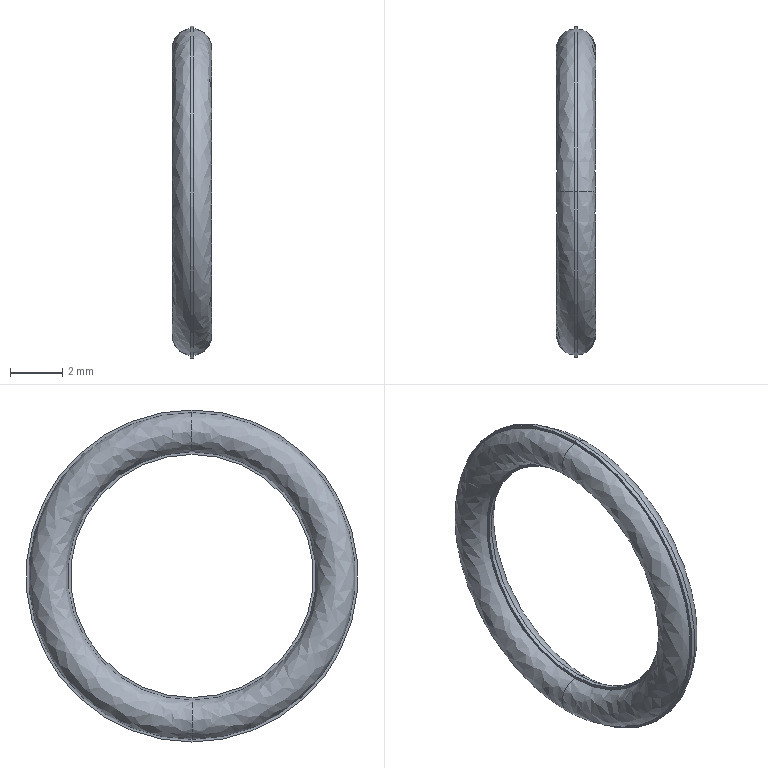Part | SolidWorks | features BaseBody 1 | 1 solid | 12 faces | box 1.5 x 12.7 x 12.7 mm | volume 62.118 mm3 | spline 4 | cylinder 4 | plane 4 | commonest cylinder face diameters 9.3 x2 12.7 x2
STEP:
#1=CARTESIAN_POINT('',(0.075,0.,-4.754));
#2=VERTEX_POINT('',#1);
#3=CARTESIAN_POINT('',(0.075,0.,4.754));
#4=VERTEX_POINT('',#3);
#5=CARTESIAN_POINT('',(0.075,0.,0.));
#6=DIRECTION('',(-1.,0.,0.));
#7=DIRECTION('',(0.,0.,-1.));
#8=AXIS2_PLACEMENT_3D('',#5,#6,#7);
#9=CIRCLE('',#8,4.754);
#10=EDGE_CURVE('',#2,#4,#9,.T.);
#11=ORIENTED_EDGE('',*,*,#10,.T.);
#12=CARTESIAN_POINT('',(0.075,0.,6.246));
#13=VERTEX_POINT('',#12);
#14=CARTESIAN_POINT('',(0.,0.,5.5));
#15=DIRECTION('',(0.,-1.,0.));
#16=DIRECTION('',(0.,0.,1.));
#17=AXIS2_PLACEMENT_3D('',#14,#15,#16);
#18=CIRCLE('',#17,0.75);
#19=EDGE_CURVE('',#4,#13,#18,.T.);
#20=ORIENTED_EDGE('',*,*,#19,.T.);
#21=CARTESIAN_POINT('',(0.075,0.,-6.246));
#22=VERTEX_POINT('',#21);
#23=CARTESIAN_POINT('',(0.075,0.,0.));
#24=DIRECTION('',(1.,0.,0.));
#25=DIRECTION('',(0.,0.,-1.));
#26=AXIS2_PLACEMENT_3D('',#23,#24,#25);
#27=CIRCLE('',#26,6.246);
#28=EDGE_CURVE('',#13,#22,#27,.T.);
#29=ORIENTED_EDGE('',*,*,#28,.T.);
#30=CARTESIAN_POINT('',(0.,0.,-5.5));
#31=DIRECTION('',(0.,1.,0.));
#32=DIRECTION('',(0.,0.,-1.));
#33=AXIS2_PLACEMENT_3D('',#30,#31,#32);
#34=CIRCLE('',#33,0.75);
#35=EDGE_CURVE('',#2,#22,#34,.T.);
#36=ORIENTED_EDGE('',*,*,#35,.F.);
#37=EDGE_LOOP('',(#11,#20,#29,#36));
#38=FACE_OUTER_BOUND('',#37,.T.);
#39=CARTESIAN_POINT('',(0.075,0.,4.754));
#40=CARTESIAN_POINT('',(0.075,-9.508,4.754));
#41=CARTESIAN_POINT('',(0.075,-9.508,-4.754));
#42=CARTESIAN_POINT('',(0.075,0.,-4.754));
#43=CARTESIAN_POINT('',(1.313,0.,4.878));
#44=CARTESIAN_POINT('',(1.313,-9.756,4.878));
#45=CARTESIAN_POINT('',(1.313,-9.756,-4.878));
#46=CARTESIAN_POINT('',(1.313,0.,-4.878));
#47=CARTESIAN_POINT('',(1.313,0.,6.122));
#48=CARTESIAN_POINT('',(1.313,-12.244,6.122));
#49=CARTESIAN_POINT('',(1.313,-12.244,-6.122));
#50=CARTESIAN_POINT('',(1.313,0.,-6.122));
#51=CARTESIAN_POINT('',(0.075,0.,6.246));
#52=CARTESIAN_POINT('',(0.075,-12.492,6.246));
#53=CARTESIAN_POINT('',(0.075,-12.492,-6.246));
#54=CARTESIAN_POINT('',(0.075,0.,-6.246));
#55=(BOUNDED_SURFACE()B_SPLINE_SURFACE(3,3,((#39,#40,#41,#42),(#43,#44,#45,#46),(#47,#48,#49,#50),(#51,#52,#53,#54)),.UNSPECIFIED.,.F.,.F.,.F.)B_SPLINE_SURFACE_WITH_KNOTS((4,4),(4,4),(0.,1.),(0.,1.),.UNSPECIFIED.)GEOMETRIC_REPRESENTATION_ITEM()RATIONAL_B_SPLINE_SURFACE(((1.,0.3333,0.3333,1.),(0.4,0.1333,0.1333,0.4),(0.4,0.1333,0.1333,0.4),(1.,0.3333,0.3333,1.)))REPRESENTATION_ITEM('')SURFACE());
#56=ADVANCED_FACE('',(#38),#55,.T.);
#57=CARTESIAN_POINT('',(-0.075,0.,6.246));
#58=VERTEX_POINT('',#57);
#59=CARTESIAN_POINT('',(-0.075,0.,-6.246));
#60=VERTEX_POINT('',#59);
#61=CARTESIAN_POINT('',(-0.075,0.,0.));
#62=DIRECTION('',(1.,0.,0.));
#63=DIRECTION('',(0.,0.,-1.));
#64=AXIS2_PLACEMENT_3D('',#61,#62,#63);
#65=CIRCLE('',#64,6.246);
#66=EDGE_CURVE('',#58,#60,#65,.T.);
#67=ORIENTED_EDGE('',*,*,#66,.F.);
#68=CARTESIAN_POINT('',(-0.075,0.,4.754));
#69=VERTEX_POINT('',#68);
#70=CARTESIAN_POINT('',(0.,0.,5.5));
#71=DIRECTION('',(0.,-1.,0.));
#72=DIRECTION('',(0.,0.,1.));
#73=AXIS2_PLACEMENT_3D('',#70,#71,#72);
#74=CIRCLE('',#73,0.75);
#75=EDGE_CURVE('',#58,#69,#74,.T.);
#76=ORIENTED_EDGE('',*,*,#75,.T.);
#77=CARTESIAN_POINT('',(-0.075,0.,-4.754));
#78=VERTEX_POINT('',#77);
#79=CARTESIAN_POINT('',(-0.075,0.,0.));
#80=DIRECTION('',(-1.,0.,0.));
#81=DIRECTION('',(0.,0.,-1.));
#82=AXIS2_PLACEMENT_3D('',#79,#80,#81);
#83=CIRCLE('',#82,4.754);
#84=EDGE_CURVE('',#78,#69,#83,.T.);
#85=ORIENTED_EDGE('',*,*,#84,.F.);
#86=CARTESIAN_POINT('',(0.,0.,-5.5));
#87=DIRECTION('',(0.,1.,0.));
#88=DIRECTION('',(0.,0.,-1.));
#89=AXIS2_PLACEMENT_3D('',#86,#87,#88);
#90=CIRCLE('',#89,0.75);
#91=EDGE_CURVE('',#60,#78,#90,.T.);
#92=ORIENTED_EDGE('',*,*,#91,.F.);
#93=EDGE_LOOP('',(#67,#76,#85,#92));
#94=FACE_OUTER_BOUND('',#93,.T.);
#95=CARTESIAN_POINT('',(-0.075,0.,6.246));
#96=CARTESIAN_POINT('',(-0.075,-12.492,6.246));
#97=CARTESIAN_POINT('',(-0.075,-12.492,-6.246));
#98=CARTESIAN_POINT('',(-0.075,0.,-6.246));
#99=CARTESIAN_POINT('',(-1.313,0.,6.122));
#100=CARTESIAN_POINT('',(-1.313,-12.244,6.122));
#101=CARTESIAN_POINT('',(-1.313,-12.244,-6.122));
#102=CARTESIAN_POINT('',(-1.313,0.,-6.122));
#103=CARTESIAN_POINT('',(-1.313,0.,4.878));
#104=CARTESIAN_POINT('',(-1.313,-9.756,4.878));
#105=CARTESIAN_POINT('',(-1.313,-9.756,-4.878));
#106=CARTESIAN_POINT('',(-1.313,0.,-4.878));
#107=CARTESIAN_POINT('',(-0.075,0.,4.754));
#108=CARTESIAN_POINT('',(-0.075,-9.508,4.754));
#109=CARTESIAN_POINT('',(-0.075,-9.508,-4.754));
#110=CARTESIAN_POINT('',(-0.075,0.,-4.754));
#111=(BOUNDED_SURFACE()B_SPLINE_SURFACE(3,3,((#95,#96,#97,#98),(#99,#100,#101,#102),(#103,#104,#105,#106),(#107,#108,#109,#110)),.UNSPECIFIED.,.F.,.F.,.F.)B_SPLINE_SURFACE_WITH_KNOTS((4,4),(4,4),(0.,1.),(0.,1.),.UNSPECIFIED.)GEOMETRIC_REPRESENTATION_ITEM()RATIONAL_B_SPLINE_SURFACE(((1.,0.3333,0.3333,1.),(0.4,0.1333,0.1333,0.4),(0.4,0.1333,0.1333,0.4),(1.,0.3333,0.3333,1.)))REPRESENTATION_ITEM('')SURFACE());
#112=ADVANCED_FACE('',(#94),#111,.T.);
#113=CARTESIAN_POINT('',(0.075,0.,-4.65));
#114=VERTEX_POINT('',#113);
#115=CARTESIAN_POINT('',(0.075,0.,4.65));
#116=VERTEX_POINT('',#115);
#117=CARTESIAN_POINT('',(0.075,0.,0.));
#118=DIRECTION('',(-1.,0.,0.));
#119=DIRECTION('',(0.,0.,1.));
#120=AXIS2_PLACEMENT_3D('',#117,#118,#119);
#121=CIRCLE('',#120,4.65);
#122=EDGE_CURVE('',#114,#116,#121,.T.);
#123=ORIENTED_EDGE('',*,*,#122,.F.);
#124=CARTESIAN_POINT('',(-0.075,0.,-4.65));
#125=VERTEX_POINT('',#124);
#126=CARTESIAN_POINT('',(1.5,0.,-4.65));
#127=DIRECTION('',(-1.,0.,0.));
#128=VECTOR('',#127,1000.);
#129=LINE('',#126,#128);
#130=EDGE_CURVE('',#114,#125,#129,.T.);
#131=ORIENTED_EDGE('',*,*,#130,.T.);
#132=CARTESIAN_POINT('',(-0.075,0.,4.65));
#133=VERTEX_POINT('',#132);
#134=CARTESIAN_POINT('',(-0.075,0.,0.));
#135=DIRECTION('',(1.,0.,0.));
#136=DIRECTION('',(0.,0.,1.));
#137=AXIS2_PLACEMENT_3D('',#134,#135,#136);
#138=CIRCLE('',#137,4.65);
#139=EDGE_CURVE('',#133,#125,#138,.T.);
#140=ORIENTED_EDGE('',*,*,#139,.F.);
#141=CARTESIAN_POINT('',(1.5,0.,4.65));
#142=DIRECTION('',(-1.,0.,0.));
#143=VECTOR('',#142,1000.);
#144=LINE('',#141,#143);
#145=EDGE_CURVE('',#116,#133,#144,.T.);
#146=ORIENTED_EDGE('',*,*,#145,.F.);
#147=EDGE_LOOP('',(#123,#131,#140,#146));
#148=FACE_OUTER_BOUND('',#147,.T.);
#149=CARTESIAN_POINT('',(1.5,0.,0.));
#150=DIRECTION('',(-1.,0.,0.));
#151=DIRECTION('',(0.,0.,1.));
#152=AXIS2_PLACEMENT_3D('',#149,#150,#151);
#153=CYLINDRICAL_SURFACE('',#152,4.65);
#154=ADVANCED_FACE('',(#148),#153,.F.);
#155=CARTESIAN_POINT('',(0.075,0.,-6.35));
#156=VERTEX_POINT('',#155);
#157=CARTESIAN_POINT('',(0.075,0.,6.35));
#158=VERTEX_POINT('',#157);
#159=CARTESIAN_POINT('',(0.075,0.,0.));
#160=DIRECTION('',(1.,0.,0.));
#161=DIRECTION('',(0.,0.,1.));
#162=AXIS2_PLACEMENT_3D('',#159,#160,#161);
#163=CIRCLE('',#162,6.35);
#164=EDGE_CURVE('',#156,#158,#163,.T.);
#165=ORIENTED_EDGE('',*,*,#164,.F.);
#166=CARTESIAN_POINT('',(-0.075,0.,-6.35));
#167=VERTEX_POINT('',#166);
#168=CARTESIAN_POINT('',(1.5,0.,-6.35));
#169=DIRECTION('',(-1.,0.,0.));
#170=VECTOR('',#169,1000.);
#171=LINE('',#168,#170);
#172=EDGE_CURVE('',#156,#167,#171,.T.);
#173=ORIENTED_EDGE('',*,*,#172,.T.);
#174=CARTESIAN_POINT('',(-0.075,0.,6.35));
#175=VERTEX_POINT('',#174);
#176=CARTESIAN_POINT('',(-0.075,0.,0.));
#177=DIRECTION('',(1.,0.,0.));
#178=DIRECTION('',(0.,0.,1.));
#179=AXIS2_PLACEMENT_3D('',#176,#177,#178);
#180=CIRCLE('',#179,6.35);
#181=EDGE_CURVE('',#167,#175,#180,.T.);
#182=ORIENTED_EDGE('',*,*,#181,.T.);
#183=CARTESIAN_POINT('',(1.5,0.,6.35));
#184=DIRECTION('',(-1.,0.,0.));
#185=VECTOR('',#184,1000.);
#186=LINE('',#183,#185);
#187=EDGE_CURVE('',#158,#175,#186,.T.);
#188=ORIENTED_EDGE('',*,*,#187,.F.);
#189=EDGE_LOOP('',(#165,#173,#182,#188));
#190=FACE_OUTER_BOUND('',#189,.T.);
#191=CARTESIAN_POINT('',(1.5,0.,0.));
#192=DIRECTION('',(-1.,0.,0.));
#193=DIRECTION('',(0.,0.,1.));
#194=AXIS2_PLACEMENT_3D('',#191,#192,#193);
#195=CYLINDRICAL_SURFACE('',#194,6.35);
#196=ADVANCED_FACE('',(#190),#195,.T.);
#197=ORIENTED_EDGE('',*,*,#19,.F.);
#198=CARTESIAN_POINT('',(0.075,0.,0.));
#199=DIRECTION('',(-1.,0.,0.));
#200=DIRECTION('',(0.,0.,-1.));
#201=AXIS2_PLACEMENT_3D('',#198,#199,#200);
#202=CIRCLE('',#201,4.754);
#203=EDGE_CURVE('',#4,#2,#202,.T.);
#204=ORIENTED_EDGE('',*,*,#203,.T.);
#205=ORIENTED_EDGE('',*,*,#35,.T.);
#206=CARTESIAN_POINT('',(0.075,0.,0.));
#207=DIRECTION('',(1.,0.,0.));
#208=DIRECTION('',(0.,0.,-1.));
#209=AXIS2_PLACEMENT_3D('',#206,#207,#208);
#210=CIRCLE('',#209,6.246);
#211=EDGE_CURVE('',#22,#13,#210,.T.);
#212=ORIENTED_EDGE('',*,*,#211,.T.);
#213=EDGE_LOOP('',(#197,#204,#205,#212));
#214=FACE_OUTER_BOUND('',#213,.T.);
#215=CARTESIAN_POINT('',(0.075,0.,-4.754));
#216=CARTESIAN_POINT('',(0.075,9.508,-4.754));
#217=CARTESIAN_POINT('',(0.075,9.508,4.754));
#218=CARTESIAN_POINT('',(0.075,0.,4.754));
#219=CARTESIAN_POINT('',(1.313,0.,-4.878));
#220=CARTESIAN_POINT('',(1.313,9.756,-4.878));
#221=CARTESIAN_POINT('',(1.313,9.756,4.878));
#222=CARTESIAN_POINT('',(1.313,0.,4.878));
#223=CARTESIAN_POINT('',(1.313,0.,-6.122));
#224=CARTESIAN_POINT('',(1.313,12.244,-6.122));
#225=CARTESIAN_POINT('',(1.313,12.244,6.122));
#226=CARTESIAN_POINT('',(1.313,0.,6.122));
#227=CARTESIAN_POINT('',(0.075,0.,-6.246));
#228=CARTESIAN_POINT('',(0.075,12.492,-6.246));
#229=CARTESIAN_POINT('',(0.075,12.492,6.246));
#230=CARTESIAN_POINT('',(0.075,0.,6.246));
#231=(BOUNDED_SURFACE()B_SPLINE_SURFACE(3,3,((#215,#216,#217,#218),(#219,#220,#221,#222),(#223,#224,#225,#226),(#227,#228,#229,#230)),.UNSPECIFIED.,.F.,.F.,.F.)B_SPLINE_SURFACE_WITH_KNOTS((4,4),(4,4),(0.,1.),(0.,1.),.UNSPECIFIED.)GEOMETRIC_REPRESENTATION_ITEM()RATIONAL_B_SPLINE_SURFACE(((1.,0.3333,0.3333,1.),(0.4,0.1333,0.1333,0.4),(0.4,0.1333,0.1333,0.4),(1.,0.3333,0.3333,1.)))REPRESENTATION_ITEM('')SURFACE());
#232=ADVANCED_FACE('',(#214),#231,.T.);
#233=CARTESIAN_POINT('',(0.075,0.,0.));
#234=DIRECTION('',(-1.,0.,0.));
#235=DIRECTION('',(0.,0.,1.));
#236=AXIS2_PLACEMENT_3D('',#233,#234,#235);
#237=CIRCLE('',#236,4.65);
#238=EDGE_CURVE('',#116,#114,#237,.T.);
#239=ORIENTED_EDGE('',*,*,#238,.T.);
#240=ORIENTED_EDGE('',*,*,#122,.T.);
#241=EDGE_LOOP('',(#239,#240));
#242=FACE_BOUND('',#241,.T.);
#243=ORIENTED_EDGE('',*,*,#10,.F.);
#244=ORIENTED_EDGE('',*,*,#203,.F.);
#245=EDGE_LOOP('',(#243,#244));
#246=FACE_OUTER_BOUND('',#245,.T.);
#247=CARTESIAN_POINT('',(0.075,4.65,0.));
#248=DIRECTION('',(1.,0.,0.));
#249=DIRECTION('',(0.,0.,-1.));
#250=AXIS2_PLACEMENT_3D('',#247,#248,#249);
#251=PLANE('',#250);
#252=ADVANCED_FACE('',(#242,#246),#251,.T.);
#253=ORIENTED_EDGE('',*,*,#211,.F.);
#254=ORIENTED_EDGE('',*,*,#28,.F.);
#255=EDGE_LOOP('',(#253,#254));
#256=FACE_BOUND('',#255,.T.);
#257=CARTESIAN_POINT('',(0.075,0.,0.));
#258=DIRECTION('',(1.,0.,0.));
#259=DIRECTION('',(0.,0.,1.));
#260=AXIS2_PLACEMENT_3D('',#257,#258,#259);
#261=CIRCLE('',#260,6.35);
#262=EDGE_CURVE('',#158,#156,#261,.T.);
#263=ORIENTED_EDGE('',*,*,#262,.T.);
#264=ORIENTED_EDGE('',*,*,#164,.T.);
#265=EDGE_LOOP('',(#263,#264));
#266=FACE_OUTER_BOUND('',#265,.T.);
#267=CARTESIAN_POINT('',(0.075,6.246,0.));
#268=DIRECTION('',(1.,0.,0.));
#269=DIRECTION('',(0.,0.,-1.));
#270=AXIS2_PLACEMENT_3D('',#267,#268,#269);
#271=PLANE('',#270);
#272=ADVANCED_FACE('',(#256,#266),#271,.T.);
#273=ORIENTED_EDGE('',*,*,#130,.F.);
#274=ORIENTED_EDGE('',*,*,#238,.F.);
#275=ORIENTED_EDGE('',*,*,#145,.T.);
#276=CARTESIAN_POINT('',(-0.075,0.,0.));
#277=DIRECTION('',(1.,0.,0.));
#278=DIRECTION('',(0.,0.,1.));
#279=AXIS2_PLACEMENT_3D('',#276,#277,#278);
#280=CIRCLE('',#279,4.65);
#281=EDGE_CURVE('',#125,#133,#280,.T.);
#282=ORIENTED_EDGE('',*,*,#281,.F.);
#283=EDGE_LOOP('',(#273,#274,#275,#282));
#284=FACE_OUTER_BOUND('',#283,.T.);
#285=CARTESIAN_POINT('',(1.5,0.,0.));
#286=DIRECTION('',(-1.,0.,0.));
#287=DIRECTION('',(0.,0.,1.));
#288=AXIS2_PLACEMENT_3D('',#285,#286,#287);
#289=CYLINDRICAL_SURFACE('',#288,4.65);
#290=ADVANCED_FACE('',(#284),#289,.F.);
#291=ORIENTED_EDGE('',*,*,#172,.F.);
#292=ORIENTED_EDGE('',*,*,#262,.F.);
#293=ORIENTED_EDGE('',*,*,#187,.T.);
#294=CARTESIAN_POINT('',(-0.075,0.,0.));
#295=DIRECTION('',(1.,0.,0.));
#296=DIRECTION('',(0.,0.,1.));
#297=AXIS2_PLACEMENT_3D('',#294,#295,#296);
#298=CIRCLE('',#297,6.35);
#299=EDGE_CURVE('',#175,#167,#298,.T.);
#300=ORIENTED_EDGE('',*,*,#299,.T.);
#301=EDGE_LOOP('',(#291,#292,#293,#300));
#302=FACE_OUTER_BOUND('',#301,.T.);
#303=CARTESIAN_POINT('',(1.5,0.,0.));
#304=DIRECTION('',(-1.,0.,0.));
#305=DIRECTION('',(0.,0.,1.));
#306=AXIS2_PLACEMENT_3D('',#303,#304,#305);
#307=CYLINDRICAL_SURFACE('',#306,6.35);
#308=ADVANCED_FACE('',(#302),#307,.T.);
#309=ORIENTED_EDGE('',*,*,#84,.T.);
#310=CARTESIAN_POINT('',(-0.075,0.,0.));
#311=DIRECTION('',(-1.,0.,0.));
#312=DIRECTION('',(0.,0.,-1.));
#313=AXIS2_PLACEMENT_3D('',#310,#311,#312);
#314=CIRCLE('',#313,4.754);
#315=EDGE_CURVE('',#69,#78,#314,.T.);
#316=ORIENTED_EDGE('',*,*,#315,.T.);
#317=EDGE_LOOP('',(#309,#316));
#318=FACE_OUTER_BOUND('',#317,.T.);
#319=ORIENTED_EDGE('',*,*,#139,.T.);
#320=ORIENTED_EDGE('',*,*,#281,.T.);
#321=EDGE_LOOP('',(#319,#320));
#322=FACE_BOUND('',#321,.T.);
#323=CARTESIAN_POINT('',(-0.075,4.754,0.));
#324=DIRECTION('',(-1.,0.,0.));
#325=DIRECTION('',(0.,0.,1.));
#326=AXIS2_PLACEMENT_3D('',#323,#324,#325);
#327=PLANE('',#326);
#328=ADVANCED_FACE('',(#318,#322),#327,.T.);
#329=ORIENTED_EDGE('',*,*,#299,.F.);
#330=ORIENTED_EDGE('',*,*,#181,.F.);
#331=EDGE_LOOP('',(#329,#330));
#332=FACE_OUTER_BOUND('',#331,.T.);
#333=CARTESIAN_POINT('',(-0.075,0.,0.));
#334=DIRECTION('',(1.,0.,0.));
#335=DIRECTION('',(0.,0.,-1.));
#336=AXIS2_PLACEMENT_3D('',#333,#334,#335);
#337=CIRCLE('',#336,6.246);
#338=EDGE_CURVE('',#60,#58,#337,.T.);
#339=ORIENTED_EDGE('',*,*,#338,.T.);
#340=ORIENTED_EDGE('',*,*,#66,.T.);
#341=EDGE_LOOP('',(#339,#340));
#342=FACE_BOUND('',#341,.T.);
#343=CARTESIAN_POINT('',(-0.075,6.35,0.));
#344=DIRECTION('',(-1.,0.,0.));
#345=DIRECTION('',(0.,0.,1.));
#346=AXIS2_PLACEMENT_3D('',#343,#344,#345);
#347=PLANE('',#346);
#348=ADVANCED_FACE('',(#332,#342),#347,.T.);
#349=ORIENTED_EDGE('',*,*,#75,.F.);
#350=ORIENTED_EDGE('',*,*,#338,.F.);
#351=ORIENTED_EDGE('',*,*,#91,.T.);
#352=ORIENTED_EDGE('',*,*,#315,.F.);
#353=EDGE_LOOP('',(#349,#350,#351,#352));
#354=FACE_OUTER_BOUND('',#353,.T.);
#355=CARTESIAN_POINT('',(-0.075,0.,-6.246));
#356=CARTESIAN_POINT('',(-0.075,12.492,-6.246));
#357=CARTESIAN_POINT('',(-0.075,12.492,6.246));
#358=CARTESIAN_POINT('',(-0.075,0.,6.246));
#359=CARTESIAN_POINT('',(-1.313,0.,-6.122));
#360=CARTESIAN_POINT('',(-1.313,12.244,-6.122));
#361=CARTESIAN_POINT('',(-1.313,12.244,6.122));
#362=CARTESIAN_POINT('',(-1.313,0.,6.122));
#363=CARTESIAN_POINT('',(-1.313,0.,-4.878));
#364=CARTESIAN_POINT('',(-1.313,9.756,-4.878));
#365=CARTESIAN_POINT('',(-1.313,9.756,4.878));
#366=CARTESIAN_POINT('',(-1.313,0.,4.878));
#367=CARTESIAN_POINT('',(-0.075,0.,-4.754));
#368=CARTESIAN_POINT('',(-0.075,9.508,-4.754));
#369=CARTESIAN_POINT('',(-0.075,9.508,4.754));
#370=CARTESIAN_POINT('',(-0.075,0.,4.754));
#371=(BOUNDED_SURFACE()B_SPLINE_SURFACE(3,3,((#355,#356,#357,#358),(#359,#360,#361,#362),(#363,#364,#365,#366),(#367,#368,#369,#370)),.UNSPECIFIED.,.F.,.F.,.F.)B_SPLINE_SURFACE_WITH_KNOTS((4,4),(4,4),(0.,1.),(0.,1.),.UNSPECIFIED.)GEOMETRIC_REPRESENTATION_ITEM()RATIONAL_B_SPLINE_SURFACE(((1.,0.3333,0.3333,1.),(0.4,0.1333,0.1333,0.4),(0.4,0.1333,0.1333,0.4),(1.,0.3333,0.3333,1.)))REPRESENTATION_ITEM('')SURFACE());
#372=ADVANCED_FACE('',(#354),#371,.T.);
#373=CLOSED_SHELL('',(#56,#112,#154,#196,#232,#252,#272,#290,#308,#328,#348,#372));
#374=MANIFOLD_SOLID_BREP('',#373);
#375=CARTESIAN_POINT('',(0.,0.,0.));
#376=DIRECTION('',(0.,0.,1.));
#377=DIRECTION('',(1.,0.,0.));
#378=AXIS2_PLACEMENT_3D('',#375,#376,#377);
#379=(LENGTH_UNIT()NAMED_UNIT(*)SI_UNIT(.MILLI.,.METRE.));
#380=UNCERTAINTY_MEASURE_WITH_UNIT(LENGTH_MEASURE(0.00001),#379,'','');
#381=(NAMED_UNIT(*)PLANE_ANGLE_UNIT()SI_UNIT($,.RADIAN.));
#382=(NAMED_UNIT(*)SI_UNIT($,.STERADIAN.)SOLID_ANGLE_UNIT());
#383=(GEOMETRIC_REPRESENTATION_CONTEXT(3)GLOBAL_UNCERTAINTY_ASSIGNED_CONTEXT((#380))GLOBAL_UNIT_ASSIGNED_CONTEXT((#379,#381,#382))REPRESENTATION_CONTEXT('',''));
#384=ADVANCED_BREP_SHAPE_REPRESENTATION('',(#374,#378),#383);